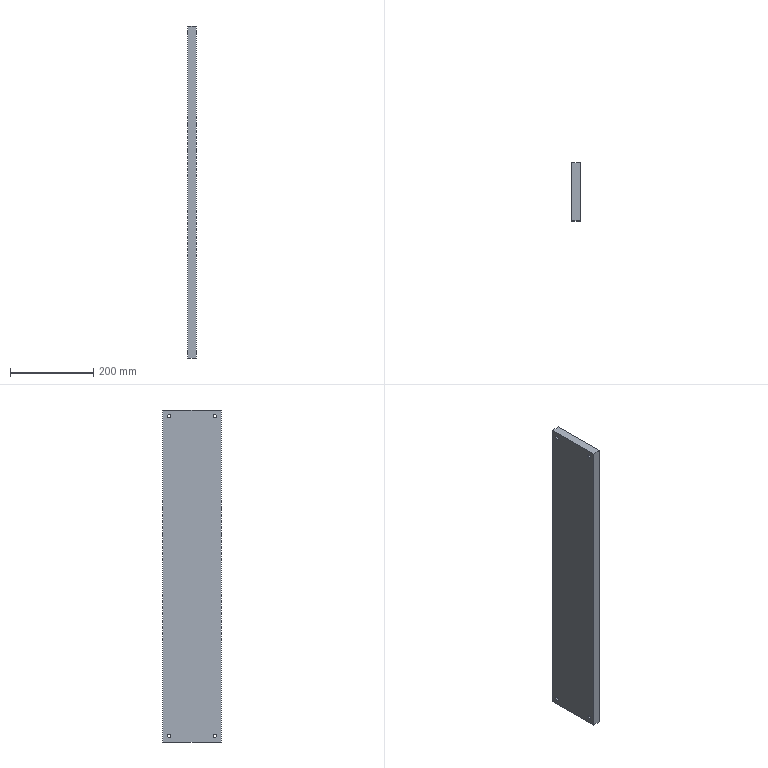Part | STEP file | A14-060 | 1 solid | 14 faces | box 20 x 140 x 800 mm | volume 2235460 mm3 | cylinder 8 | plane 6 | commonest cylinder face diameters 8.5 x8
STEP:
#1=CARTESIAN_POINT('',(0.,0.,0.));
#2=DIRECTION('',(0.,0.,1.));
#3=DIRECTION('',(1.,0.,0.));
#4=AXIS2_PLACEMENT_3D('',#1,#2,#3);
#5=CARTESIAN_POINT('',(-10.,55.,380.75));
#6=VERTEX_POINT('',#5);
#7=CARTESIAN_POINT('',(10.,55.,380.75));
#8=VERTEX_POINT('',#7);
#9=CARTESIAN_POINT('',(-10.,55.,380.75));
#10=DIRECTION('',(1.,0.,0.));
#11=VECTOR('',#10,1.);
#12=LINE('',#9,#11);
#13=CARTESIAN_POINT('',(-10.,55.,385.));
#14=DIRECTION('',(1.,0.,0.));
#15=DIRECTION('',(0.,0.,-1.));
#16=AXIS2_PLACEMENT_3D('',#13,#14,#15);
#17=CYLINDRICAL_SURFACE('',#16,4.25);
#18=CARTESIAN_POINT('',(6.283,0.));
#19=DIRECTION('',(0.,1.));
#20=VECTOR('',#19,1.);
#21=LINE('',#18,#20);
#22=(GEOMETRIC_REPRESENTATION_CONTEXT(2)PARAMETRIC_REPRESENTATION_CONTEXT()REPRESENTATION_CONTEXT('',''));
#23=DEFINITIONAL_REPRESENTATION('',(#21),#22);
#24=PCURVE('',#17,#23);
#25=CARTESIAN_POINT('',(-10.,55.,385.));
#26=DIRECTION('',(1.,0.,0.));
#27=DIRECTION('',(0.,0.,-1.));
#28=AXIS2_PLACEMENT_3D('',#25,#26,#27);
#29=CYLINDRICAL_SURFACE('',#28,4.25);
#30=CARTESIAN_POINT('',(0.,0.));
#31=DIRECTION('',(0.,1.));
#32=VECTOR('',#31,1.);
#33=LINE('',#30,#32);
#34=(GEOMETRIC_REPRESENTATION_CONTEXT(2)PARAMETRIC_REPRESENTATION_CONTEXT()REPRESENTATION_CONTEXT('',''));
#35=DEFINITIONAL_REPRESENTATION('',(#33),#34);
#36=PCURVE('',#29,#35);
#37=SURFACE_CURVE('',#12,(#24,#36),.PCURVE_S1.);
#38=EDGE_CURVE('',#6,#8,#37,.T.);
#39=ORIENTED_EDGE('',*,*,#38,.T.);
#40=CARTESIAN_POINT('',(10.,55.,389.25));
#41=VERTEX_POINT('',#40);
#42=CARTESIAN_POINT('',(10.,55.,385.));
#43=DIRECTION('',(1.,0.,0.));
#44=DIRECTION('',(0.,0.,-1.));
#45=AXIS2_PLACEMENT_3D('',#42,#43,#44);
#46=CIRCLE('',#45,4.25);
#47=CARTESIAN_POINT('',(0.,20.));
#48=DIRECTION('',(1.,0.));
#49=VECTOR('',#48,1.);
#50=LINE('',#47,#49);
#51=(GEOMETRIC_REPRESENTATION_CONTEXT(2)PARAMETRIC_REPRESENTATION_CONTEXT()REPRESENTATION_CONTEXT('',''));
#52=DEFINITIONAL_REPRESENTATION('',(#50),#51);
#53=PCURVE('',#17,#52);
#54=CARTESIAN_POINT('',(10.,0.,0.));
#55=DIRECTION('',(1.,0.,0.));
#56=DIRECTION('',(0.,0.,-1.));
#57=AXIS2_PLACEMENT_3D('',#54,#55,#56);
#58=PLANE('',#57);
#59=CARTESIAN_POINT('',(-385.,55.));
#60=DIRECTION('',(1.,0.));
#61=AXIS2_PLACEMENT_2D('',#59,#60);
#62=CIRCLE('',#61,4.25);
#63=(GEOMETRIC_REPRESENTATION_CONTEXT(2)PARAMETRIC_REPRESENTATION_CONTEXT()REPRESENTATION_CONTEXT('',''));
#64=DEFINITIONAL_REPRESENTATION('',(#62),#63);
#65=PCURVE('',#58,#64);
#66=SURFACE_CURVE('',#46,(#53,#65),.PCURVE_S1.);
#67=EDGE_CURVE('',#41,#8,#66,.T.);
#68=ORIENTED_EDGE('',*,*,#67,.F.);
#69=CARTESIAN_POINT('',(-10.,55.,389.25));
#70=VERTEX_POINT('',#69);
#71=CARTESIAN_POINT('',(-10.,55.,389.25));
#72=DIRECTION('',(1.,0.,0.));
#73=VECTOR('',#72,1.);
#74=LINE('',#71,#73);
#75=CARTESIAN_POINT('',(3.142,0.));
#76=DIRECTION('',(0.,1.));
#77=VECTOR('',#76,1.);
#78=LINE('',#75,#77);
#79=(GEOMETRIC_REPRESENTATION_CONTEXT(2)PARAMETRIC_REPRESENTATION_CONTEXT()REPRESENTATION_CONTEXT('',''));
#80=DEFINITIONAL_REPRESENTATION('',(#78),#79);
#81=PCURVE('',#17,#80);
#82=CARTESIAN_POINT('',(3.142,0.));
#83=DIRECTION('',(0.,1.));
#84=VECTOR('',#83,1.);
#85=LINE('',#82,#84);
#86=(GEOMETRIC_REPRESENTATION_CONTEXT(2)PARAMETRIC_REPRESENTATION_CONTEXT()REPRESENTATION_CONTEXT('',''));
#87=DEFINITIONAL_REPRESENTATION('',(#85),#86);
#88=PCURVE('',#29,#87);
#89=SURFACE_CURVE('',#74,(#81,#88),.PCURVE_S1.);
#90=EDGE_CURVE('',#70,#41,#89,.T.);
#91=ORIENTED_EDGE('',*,*,#90,.F.);
#92=CARTESIAN_POINT('',(-10.,55.,385.));
#93=DIRECTION('',(1.,0.,0.));
#94=DIRECTION('',(0.,0.,-1.));
#95=AXIS2_PLACEMENT_3D('',#92,#93,#94);
#96=CIRCLE('',#95,4.25);
#97=CARTESIAN_POINT('',(0.,0.));
#98=DIRECTION('',(1.,0.));
#99=VECTOR('',#98,1.);
#100=LINE('',#97,#99);
#101=(GEOMETRIC_REPRESENTATION_CONTEXT(2)PARAMETRIC_REPRESENTATION_CONTEXT()REPRESENTATION_CONTEXT('',''));
#102=DEFINITIONAL_REPRESENTATION('',(#100),#101);
#103=PCURVE('',#17,#102);
#104=CARTESIAN_POINT('',(-10.,0.,0.));
#105=DIRECTION('',(1.,0.,0.));
#106=DIRECTION('',(0.,0.,-1.));
#107=AXIS2_PLACEMENT_3D('',#104,#105,#106);
#108=PLANE('',#107);
#109=CARTESIAN_POINT('',(-385.,55.));
#110=DIRECTION('',(1.,0.));
#111=AXIS2_PLACEMENT_2D('',#109,#110);
#112=CIRCLE('',#111,4.25);
#113=(GEOMETRIC_REPRESENTATION_CONTEXT(2)PARAMETRIC_REPRESENTATION_CONTEXT()REPRESENTATION_CONTEXT('',''));
#114=DEFINITIONAL_REPRESENTATION('',(#112),#113);
#115=PCURVE('',#108,#114);
#116=SURFACE_CURVE('',#96,(#103,#115),.PCURVE_S1.);
#117=EDGE_CURVE('',#70,#6,#116,.T.);
#118=ORIENTED_EDGE('',*,*,#117,.T.);
#119=EDGE_LOOP('',(#39,#68,#91,#118));
#120=FACE_BOUND('',#119,.F.);
#121=ADVANCED_FACE('',(#120),#17,.F.);
#122=CARTESIAN_POINT('',(-10.,-55.,380.75));
#123=VERTEX_POINT('',#122);
#124=CARTESIAN_POINT('',(10.,-55.,380.75));
#125=VERTEX_POINT('',#124);
#126=CARTESIAN_POINT('',(-10.,-55.,380.75));
#127=DIRECTION('',(1.,0.,0.));
#128=VECTOR('',#127,1.);
#129=LINE('',#126,#128);
#130=CARTESIAN_POINT('',(-10.,-55.,385.));
#131=DIRECTION('',(1.,0.,0.));
#132=DIRECTION('',(0.,0.,-1.));
#133=AXIS2_PLACEMENT_3D('',#130,#131,#132);
#134=CYLINDRICAL_SURFACE('',#133,4.25);
#135=CARTESIAN_POINT('',(6.283,0.));
#136=DIRECTION('',(0.,1.));
#137=VECTOR('',#136,1.);
#138=LINE('',#135,#137);
#139=(GEOMETRIC_REPRESENTATION_CONTEXT(2)PARAMETRIC_REPRESENTATION_CONTEXT()REPRESENTATION_CONTEXT('',''));
#140=DEFINITIONAL_REPRESENTATION('',(#138),#139);
#141=PCURVE('',#134,#140);
#142=CARTESIAN_POINT('',(-10.,-55.,385.));
#143=DIRECTION('',(1.,0.,0.));
#144=DIRECTION('',(0.,0.,-1.));
#145=AXIS2_PLACEMENT_3D('',#142,#143,#144);
#146=CYLINDRICAL_SURFACE('',#145,4.25);
#147=CARTESIAN_POINT('',(0.,0.));
#148=DIRECTION('',(0.,1.));
#149=VECTOR('',#148,1.);
#150=LINE('',#147,#149);
#151=(GEOMETRIC_REPRESENTATION_CONTEXT(2)PARAMETRIC_REPRESENTATION_CONTEXT()REPRESENTATION_CONTEXT('',''));
#152=DEFINITIONAL_REPRESENTATION('',(#150),#151);
#153=PCURVE('',#146,#152);
#154=SURFACE_CURVE('',#129,(#141,#153),.PCURVE_S1.);
#155=EDGE_CURVE('',#123,#125,#154,.T.);
#156=ORIENTED_EDGE('',*,*,#155,.T.);
#157=CARTESIAN_POINT('',(10.,-55.,389.25));
#158=VERTEX_POINT('',#157);
#159=CARTESIAN_POINT('',(10.,-55.,385.));
#160=DIRECTION('',(1.,0.,0.));
#161=DIRECTION('',(0.,0.,-1.));
#162=AXIS2_PLACEMENT_3D('',#159,#160,#161);
#163=CIRCLE('',#162,4.25);
#164=CARTESIAN_POINT('',(0.,20.));
#165=DIRECTION('',(1.,0.));
#166=VECTOR('',#165,1.);
#167=LINE('',#164,#166);
#168=(GEOMETRIC_REPRESENTATION_CONTEXT(2)PARAMETRIC_REPRESENTATION_CONTEXT()REPRESENTATION_CONTEXT('',''));
#169=DEFINITIONAL_REPRESENTATION('',(#167),#168);
#170=PCURVE('',#134,#169);
#171=CARTESIAN_POINT('',(-385.,-55.));
#172=DIRECTION('',(1.,0.));
#173=AXIS2_PLACEMENT_2D('',#171,#172);
#174=CIRCLE('',#173,4.25);
#175=(GEOMETRIC_REPRESENTATION_CONTEXT(2)PARAMETRIC_REPRESENTATION_CONTEXT()REPRESENTATION_CONTEXT('',''));
#176=DEFINITIONAL_REPRESENTATION('',(#174),#175);
#177=PCURVE('',#58,#176);
#178=SURFACE_CURVE('',#163,(#170,#177),.PCURVE_S1.);
#179=EDGE_CURVE('',#158,#125,#178,.T.);
#180=ORIENTED_EDGE('',*,*,#179,.F.);
#181=CARTESIAN_POINT('',(-10.,-55.,389.25));
#182=VERTEX_POINT('',#181);
#183=CARTESIAN_POINT('',(-10.,-55.,389.25));
#184=DIRECTION('',(1.,0.,0.));
#185=VECTOR('',#184,1.);
#186=LINE('',#183,#185);
#187=CARTESIAN_POINT('',(3.142,0.));
#188=DIRECTION('',(0.,1.));
#189=VECTOR('',#188,1.);
#190=LINE('',#187,#189);
#191=(GEOMETRIC_REPRESENTATION_CONTEXT(2)PARAMETRIC_REPRESENTATION_CONTEXT()REPRESENTATION_CONTEXT('',''));
#192=DEFINITIONAL_REPRESENTATION('',(#190),#191);
#193=PCURVE('',#134,#192);
#194=CARTESIAN_POINT('',(3.142,0.));
#195=DIRECTION('',(0.,1.));
#196=VECTOR('',#195,1.);
#197=LINE('',#194,#196);
#198=(GEOMETRIC_REPRESENTATION_CONTEXT(2)PARAMETRIC_REPRESENTATION_CONTEXT()REPRESENTATION_CONTEXT('',''));
#199=DEFINITIONAL_REPRESENTATION('',(#197),#198);
#200=PCURVE('',#146,#199);
#201=SURFACE_CURVE('',#186,(#193,#200),.PCURVE_S1.);
#202=EDGE_CURVE('',#182,#158,#201,.T.);
#203=ORIENTED_EDGE('',*,*,#202,.F.);
#204=CARTESIAN_POINT('',(-10.,-55.,385.));
#205=DIRECTION('',(1.,0.,0.));
#206=DIRECTION('',(0.,0.,-1.));
#207=AXIS2_PLACEMENT_3D('',#204,#205,#206);
#208=CIRCLE('',#207,4.25);
#209=CARTESIAN_POINT('',(0.,0.));
#210=DIRECTION('',(1.,0.));
#211=VECTOR('',#210,1.);
#212=LINE('',#209,#211);
#213=(GEOMETRIC_REPRESENTATION_CONTEXT(2)PARAMETRIC_REPRESENTATION_CONTEXT()REPRESENTATION_CONTEXT('',''));
#214=DEFINITIONAL_REPRESENTATION('',(#212),#213);
#215=PCURVE('',#134,#214);
#216=CARTESIAN_POINT('',(-385.,-55.));
#217=DIRECTION('',(1.,0.));
#218=AXIS2_PLACEMENT_2D('',#216,#217);
#219=CIRCLE('',#218,4.25);
#220=(GEOMETRIC_REPRESENTATION_CONTEXT(2)PARAMETRIC_REPRESENTATION_CONTEXT()REPRESENTATION_CONTEXT('',''));
#221=DEFINITIONAL_REPRESENTATION('',(#219),#220);
#222=PCURVE('',#108,#221);
#223=SURFACE_CURVE('',#208,(#215,#222),.PCURVE_S1.);
#224=EDGE_CURVE('',#182,#123,#223,.T.);
#225=ORIENTED_EDGE('',*,*,#224,.T.);
#226=EDGE_LOOP('',(#156,#180,#203,#225));
#227=FACE_BOUND('',#226,.F.);
#228=ADVANCED_FACE('',(#227),#134,.F.);
#229=CARTESIAN_POINT('',(-10.,-55.,-389.25));
#230=VERTEX_POINT('',#229);
#231=CARTESIAN_POINT('',(10.,-55.,-389.25));
#232=VERTEX_POINT('',#231);
#233=CARTESIAN_POINT('',(-10.,-55.,-389.25));
#234=DIRECTION('',(1.,0.,0.));
#235=VECTOR('',#234,1.);
#236=LINE('',#233,#235);
#237=CARTESIAN_POINT('',(-10.,-55.,-385.));
#238=DIRECTION('',(1.,0.,0.));
#239=DIRECTION('',(0.,0.,-1.));
#240=AXIS2_PLACEMENT_3D('',#237,#238,#239);
#241=CYLINDRICAL_SURFACE('',#240,4.25);
#242=CARTESIAN_POINT('',(6.283,0.));
#243=DIRECTION('',(0.,1.));
#244=VECTOR('',#243,1.);
#245=LINE('',#242,#244);
#246=(GEOMETRIC_REPRESENTATION_CONTEXT(2)PARAMETRIC_REPRESENTATION_CONTEXT()REPRESENTATION_CONTEXT('',''));
#247=DEFINITIONAL_REPRESENTATION('',(#245),#246);
#248=PCURVE('',#241,#247);
#249=CARTESIAN_POINT('',(-10.,-55.,-385.));
#250=DIRECTION('',(1.,0.,0.));
#251=DIRECTION('',(0.,0.,-1.));
#252=AXIS2_PLACEMENT_3D('',#249,#250,#251);
#253=CYLINDRICAL_SURFACE('',#252,4.25);
#254=CARTESIAN_POINT('',(0.,0.));
#255=DIRECTION('',(0.,1.));
#256=VECTOR('',#255,1.);
#257=LINE('',#254,#256);
#258=(GEOMETRIC_REPRESENTATION_CONTEXT(2)PARAMETRIC_REPRESENTATION_CONTEXT()REPRESENTATION_CONTEXT('',''));
#259=DEFINITIONAL_REPRESENTATION('',(#257),#258);
#260=PCURVE('',#253,#259);
#261=SURFACE_CURVE('',#236,(#248,#260),.PCURVE_S1.);
#262=EDGE_CURVE('',#230,#232,#261,.T.);
#263=ORIENTED_EDGE('',*,*,#262,.T.);
#264=CARTESIAN_POINT('',(10.,-55.,-380.75));
#265=VERTEX_POINT('',#264);
#266=CARTESIAN_POINT('',(10.,-55.,-385.));
#267=DIRECTION('',(1.,0.,0.));
#268=DIRECTION('',(0.,0.,-1.));
#269=AXIS2_PLACEMENT_3D('',#266,#267,#268);
#270=CIRCLE('',#269,4.25);
#271=CARTESIAN_POINT('',(0.,20.));
#272=DIRECTION('',(1.,0.));
#273=VECTOR('',#272,1.);
#274=LINE('',#271,#273);
#275=(GEOMETRIC_REPRESENTATION_CONTEXT(2)PARAMETRIC_REPRESENTATION_CONTEXT()REPRESENTATION_CONTEXT('',''));
#276=DEFINITIONAL_REPRESENTATION('',(#274),#275);
#277=PCURVE('',#241,#276);
#278=CARTESIAN_POINT('',(385.,-55.));
#279=DIRECTION('',(1.,0.));
#280=AXIS2_PLACEMENT_2D('',#278,#279);
#281=CIRCLE('',#280,4.25);
#282=(GEOMETRIC_REPRESENTATION_CONTEXT(2)PARAMETRIC_REPRESENTATION_CONTEXT()REPRESENTATION_CONTEXT('',''));
#283=DEFINITIONAL_REPRESENTATION('',(#281),#282);
#284=PCURVE('',#58,#283);
#285=SURFACE_CURVE('',#270,(#277,#284),.PCURVE_S1.);
#286=EDGE_CURVE('',#265,#232,#285,.T.);
#287=ORIENTED_EDGE('',*,*,#286,.F.);
#288=CARTESIAN_POINT('',(-10.,-55.,-380.75));
#289=VERTEX_POINT('',#288);
#290=CARTESIAN_POINT('',(-10.,-55.,-380.75));
#291=DIRECTION('',(1.,0.,0.));
#292=VECTOR('',#291,1.);
#293=LINE('',#290,#292);
#294=CARTESIAN_POINT('',(3.142,0.));
#295=DIRECTION('',(0.,1.));
#296=VECTOR('',#295,1.);
#297=LINE('',#294,#296);
#298=(GEOMETRIC_REPRESENTATION_CONTEXT(2)PARAMETRIC_REPRESENTATION_CONTEXT()REPRESENTATION_CONTEXT('',''));
#299=DEFINITIONAL_REPRESENTATION('',(#297),#298);
#300=PCURVE('',#241,#299);
#301=CARTESIAN_POINT('',(3.142,0.));
#302=DIRECTION('',(0.,1.));
#303=VECTOR('',#302,1.);
#304=LINE('',#301,#303);
#305=(GEOMETRIC_REPRESENTATION_CONTEXT(2)PARAMETRIC_REPRESENTATION_CONTEXT()REPRESENTATION_CONTEXT('',''));
#306=DEFINITIONAL_REPRESENTATION('',(#304),#305);
#307=PCURVE('',#253,#306);
#308=SURFACE_CURVE('',#293,(#300,#307),.PCURVE_S1.);
#309=EDGE_CURVE('',#289,#265,#308,.T.);
#310=ORIENTED_EDGE('',*,*,#309,.F.);
#311=CARTESIAN_POINT('',(-10.,-55.,-385.));
#312=DIRECTION('',(1.,0.,0.));
#313=DIRECTION('',(0.,0.,-1.));
#314=AXIS2_PLACEMENT_3D('',#311,#312,#313);
#315=CIRCLE('',#314,4.25);
#316=CARTESIAN_POINT('',(0.,0.));
#317=DIRECTION('',(1.,0.));
#318=VECTOR('',#317,1.);
#319=LINE('',#316,#318);
#320=(GEOMETRIC_REPRESENTATION_CONTEXT(2)PARAMETRIC_REPRESENTATION_CONTEXT()REPRESENTATION_CONTEXT('',''));
#321=DEFINITIONAL_REPRESENTATION('',(#319),#320);
#322=PCURVE('',#241,#321);
#323=CARTESIAN_POINT('',(385.,-55.));
#324=DIRECTION('',(1.,0.));
#325=AXIS2_PLACEMENT_2D('',#323,#324);
#326=CIRCLE('',#325,4.25);
#327=(GEOMETRIC_REPRESENTATION_CONTEXT(2)PARAMETRIC_REPRESENTATION_CONTEXT()REPRESENTATION_CONTEXT('',''));
#328=DEFINITIONAL_REPRESENTATION('',(#326),#327);
#329=PCURVE('',#108,#328);
#330=SURFACE_CURVE('',#315,(#322,#329),.PCURVE_S1.);
#331=EDGE_CURVE('',#289,#230,#330,.T.);
#332=ORIENTED_EDGE('',*,*,#331,.T.);
#333=EDGE_LOOP('',(#263,#287,#310,#332));
#334=FACE_BOUND('',#333,.F.);
#335=ADVANCED_FACE('',(#334),#241,.F.);
#336=CARTESIAN_POINT('',(-10.,55.,-389.25));
#337=VERTEX_POINT('',#336);
#338=CARTESIAN_POINT('',(10.,55.,-389.25));
#339=VERTEX_POINT('',#338);
#340=CARTESIAN_POINT('',(-10.,55.,-389.25));
#341=DIRECTION('',(1.,0.,0.));
#342=VECTOR('',#341,1.);
#343=LINE('',#340,#342);
#344=CARTESIAN_POINT('',(-10.,55.,-385.));
#345=DIRECTION('',(1.,0.,0.));
#346=DIRECTION('',(0.,0.,-1.));
#347=AXIS2_PLACEMENT_3D('',#344,#345,#346);
#348=CYLINDRICAL_SURFACE('',#347,4.25);
#349=CARTESIAN_POINT('',(6.283,0.));
#350=DIRECTION('',(0.,1.));
#351=VECTOR('',#350,1.);
#352=LINE('',#349,#351);
#353=(GEOMETRIC_REPRESENTATION_CONTEXT(2)PARAMETRIC_REPRESENTATION_CONTEXT()REPRESENTATION_CONTEXT('',''));
#354=DEFINITIONAL_REPRESENTATION('',(#352),#353);
#355=PCURVE('',#348,#354);
#356=CARTESIAN_POINT('',(-10.,55.,-385.));
#357=DIRECTION('',(1.,0.,0.));
#358=DIRECTION('',(0.,0.,-1.));
#359=AXIS2_PLACEMENT_3D('',#356,#357,#358);
#360=CYLINDRICAL_SURFACE('',#359,4.25);
#361=CARTESIAN_POINT('',(0.,0.));
#362=DIRECTION('',(0.,1.));
#363=VECTOR('',#362,1.);
#364=LINE('',#361,#363);
#365=(GEOMETRIC_REPRESENTATION_CONTEXT(2)PARAMETRIC_REPRESENTATION_CONTEXT()REPRESENTATION_CONTEXT('',''));
#366=DEFINITIONAL_REPRESENTATION('',(#364),#365);
#367=PCURVE('',#360,#366);
#368=SURFACE_CURVE('',#343,(#355,#367),.PCURVE_S1.);
#369=EDGE_CURVE('',#337,#339,#368,.T.);
#370=ORIENTED_EDGE('',*,*,#369,.T.);
#371=CARTESIAN_POINT('',(10.,55.,-380.75));
#372=VERTEX_POINT('',#371);
#373=CARTESIAN_POINT('',(10.,55.,-385.));
#374=DIRECTION('',(1.,0.,0.));
#375=DIRECTION('',(0.,0.,-1.));
#376=AXIS2_PLACEMENT_3D('',#373,#374,#375);
#377=CIRCLE('',#376,4.25);
#378=CARTESIAN_POINT('',(0.,20.));
#379=DIRECTION('',(1.,0.));
#380=VECTOR('',#379,1.);
#381=LINE('',#378,#380);
#382=(GEOMETRIC_REPRESENTATION_CONTEXT(2)PARAMETRIC_REPRESENTATION_CONTEXT()REPRESENTATION_CONTEXT('',''));
#383=DEFINITIONAL_REPRESENTATION('',(#381),#382);
#384=PCURVE('',#348,#383);
#385=CARTESIAN_POINT('',(385.,55.));
#386=DIRECTION('',(1.,0.));
#387=AXIS2_PLACEMENT_2D('',#385,#386);
#388=CIRCLE('',#387,4.25);
#389=(GEOMETRIC_REPRESENTATION_CONTEXT(2)PARAMETRIC_REPRESENTATION_CONTEXT()REPRESENTATION_CONTEXT('',''));
#390=DEFINITIONAL_REPRESENTATION('',(#388),#389);
#391=PCURVE('',#58,#390);
#392=SURFACE_CURVE('',#377,(#384,#391),.PCURVE_S1.);
#393=EDGE_CURVE('',#372,#339,#392,.T.);
#394=ORIENTED_EDGE('',*,*,#393,.F.);
#395=CARTESIAN_POINT('',(-10.,55.,-380.75));
#396=VERTEX_POINT('',#395);
#397=CARTESIAN_POINT('',(-10.,55.,-380.75));
#398=DIRECTION('',(1.,0.,0.));
#399=VECTOR('',#398,1.);
#400=LINE('',#397,#399);
#401=CARTESIAN_POINT('',(3.142,0.));
#402=DIRECTION('',(0.,1.));
#403=VECTOR('',#402,1.);
#404=LINE('',#401,#403);
#405=(GEOMETRIC_REPRESENTATION_CONTEXT(2)PARAMETRIC_REPRESENTATION_CONTEXT()REPRESENTATION_CONTEXT('',''));
#406=DEFINITIONAL_REPRESENTATION('',(#404),#405);
#407=PCURVE('',#348,#406);
#408=CARTESIAN_POINT('',(3.142,0.));
#409=DIRECTION('',(0.,1.));
#410=VECTOR('',#409,1.);
#411=LINE('',#408,#410);
#412=(GEOMETRIC_REPRESENTATION_CONTEXT(2)PARAMETRIC_REPRESENTATION_CONTEXT()REPRESENTATION_CONTEXT('',''));
#413=DEFINITIONAL_REPRESENTATION('',(#411),#412);
#414=PCURVE('',#360,#413);
#415=SURFACE_CURVE('',#400,(#407,#414),.PCURVE_S1.);
#416=EDGE_CURVE('',#396,#372,#415,.T.);
#417=ORIENTED_EDGE('',*,*,#416,.F.);
#418=CARTESIAN_POINT('',(-10.,55.,-385.));
#419=DIRECTION('',(1.,0.,0.));
#420=DIRECTION('',(0.,0.,-1.));
#421=AXIS2_PLACEMENT_3D('',#418,#419,#420);
#422=CIRCLE('',#421,4.25);
#423=CARTESIAN_POINT('',(0.,0.));
#424=DIRECTION('',(1.,0.));
#425=VECTOR('',#424,1.);
#426=LINE('',#423,#425);
#427=(GEOMETRIC_REPRESENTATION_CONTEXT(2)PARAMETRIC_REPRESENTATION_CONTEXT()REPRESENTATION_CONTEXT('',''));
#428=DEFINITIONAL_REPRESENTATION('',(#426),#427);
#429=PCURVE('',#348,#428);
#430=CARTESIAN_POINT('',(385.,55.));
#431=DIRECTION('',(1.,0.));
#432=AXIS2_PLACEMENT_2D('',#430,#431);
#433=CIRCLE('',#432,4.25);
#434=(GEOMETRIC_REPRESENTATION_CONTEXT(2)PARAMETRIC_REPRESENTATION_CONTEXT()REPRESENTATION_CONTEXT('',''));
#435=DEFINITIONAL_REPRESENTATION('',(#433),#434);
#436=PCURVE('',#108,#435);
#437=SURFACE_CURVE('',#422,(#429,#436),.PCURVE_S1.);
#438=EDGE_CURVE('',#396,#337,#437,.T.);
#439=ORIENTED_EDGE('',*,*,#438,.T.);
#440=EDGE_LOOP('',(#370,#394,#417,#439));
#441=FACE_BOUND('',#440,.F.);
#442=ADVANCED_FACE('',(#441),#348,.F.);
#443=CARTESIAN_POINT('',(-10.,-70.,-400.));
#444=VERTEX_POINT('',#443);
#445=CARTESIAN_POINT('',(-10.,70.,-400.));
#446=VERTEX_POINT('',#445);
#447=CARTESIAN_POINT('',(-10.,70.,-400.));
#448=DIRECTION('',(0.,1.,0.));
#449=VECTOR('',#448,1.);
#450=LINE('',#447,#449);
#451=CARTESIAN_POINT('',(10.,70.,-400.));
#452=DIRECTION('',(0.,0.,1.));
#453=DIRECTION('',(1.,0.,0.));
#454=AXIS2_PLACEMENT_3D('',#451,#452,#453);
#455=PLANE('',#454);
#456=CARTESIAN_POINT('',(-20.,0.));
#457=DIRECTION('',(0.,1.));
#458=VECTOR('',#457,1.);
#459=LINE('',#456,#458);
#460=(GEOMETRIC_REPRESENTATION_CONTEXT(2)PARAMETRIC_REPRESENTATION_CONTEXT()REPRESENTATION_CONTEXT('',''));
#461=DEFINITIONAL_REPRESENTATION('',(#459),#460);
#462=PCURVE('',#455,#461);
#463=CARTESIAN_POINT('',(400.,70.));
#464=DIRECTION('',(0.,1.));
#465=VECTOR('',#464,1.);
#466=LINE('',#463,#465);
#467=(GEOMETRIC_REPRESENTATION_CONTEXT(2)PARAMETRIC_REPRESENTATION_CONTEXT()REPRESENTATION_CONTEXT('',''));
#468=DEFINITIONAL_REPRESENTATION('',(#466),#467);
#469=PCURVE('',#108,#468);
#470=SURFACE_CURVE('',#450,(#462,#469),.PCURVE_S1.);
#471=EDGE_CURVE('',#444,#446,#470,.T.);
#472=ORIENTED_EDGE('',*,*,#471,.T.);
#473=CARTESIAN_POINT('',(10.,70.,-400.));
#474=VERTEX_POINT('',#473);
#475=CARTESIAN_POINT('',(10.,70.,-400.));
#476=DIRECTION('',(-1.,0.,0.));
#477=VECTOR('',#476,1.);
#478=LINE('',#475,#477);
#479=CARTESIAN_POINT('',(0.,0.));
#480=DIRECTION('',(-1.,0.));
#481=VECTOR('',#480,1.);
#482=LINE('',#479,#481);
#483=(GEOMETRIC_REPRESENTATION_CONTEXT(2)PARAMETRIC_REPRESENTATION_CONTEXT()REPRESENTATION_CONTEXT('',''));
#484=DEFINITIONAL_REPRESENTATION('',(#482),#483);
#485=PCURVE('',#455,#484);
#486=CARTESIAN_POINT('',(10.,70.,400.));
#487=DIRECTION('',(0.,-1.,0.));
#488=DIRECTION('',(0.,0.,-1.));
#489=AXIS2_PLACEMENT_3D('',#486,#487,#488);
#490=PLANE('',#489);
#491=CARTESIAN_POINT('',(800.,0.));
#492=DIRECTION('',(0.,-1.));
#493=VECTOR('',#492,1.);
#494=LINE('',#491,#493);
#495=(GEOMETRIC_REPRESENTATION_CONTEXT(2)PARAMETRIC_REPRESENTATION_CONTEXT()REPRESENTATION_CONTEXT('',''));
#496=DEFINITIONAL_REPRESENTATION('',(#494),#495);
#497=PCURVE('',#490,#496);
#498=SURFACE_CURVE('',#478,(#485,#497),.PCURVE_S1.);
#499=EDGE_CURVE('',#474,#446,#498,.T.);
#500=ORIENTED_EDGE('',*,*,#499,.F.);
#501=CARTESIAN_POINT('',(10.,-70.,-400.));
#502=VERTEX_POINT('',#501);
#503=CARTESIAN_POINT('',(10.,70.,-400.));
#504=DIRECTION('',(0.,1.,0.));
#505=VECTOR('',#504,1.);
#506=LINE('',#503,#505);
#507=CARTESIAN_POINT('',(0.,0.));
#508=DIRECTION('',(0.,1.));
#509=VECTOR('',#508,1.);
#510=LINE('',#507,#509);
#511=(GEOMETRIC_REPRESENTATION_CONTEXT(2)PARAMETRIC_REPRESENTATION_CONTEXT()REPRESENTATION_CONTEXT('',''));
#512=DEFINITIONAL_REPRESENTATION('',(#510),#511);
#513=PCURVE('',#455,#512);
#514=CARTESIAN_POINT('',(400.,70.));
#515=DIRECTION('',(0.,1.));
#516=VECTOR('',#515,1.);
#517=LINE('',#514,#516);
#518=(GEOMETRIC_REPRESENTATION_CONTEXT(2)PARAMETRIC_REPRESENTATION_CONTEXT()REPRESENTATION_CONTEXT('',''));
#519=DEFINITIONAL_REPRESENTATION('',(#517),#518);
#520=PCURVE('',#58,#519);
#521=SURFACE_CURVE('',#506,(#513,#520),.PCURVE_S1.);
#522=EDGE_CURVE('',#502,#474,#521,.T.);
#523=ORIENTED_EDGE('',*,*,#522,.F.);
#524=CARTESIAN_POINT('',(10.,-70.,-400.));
#525=DIRECTION('',(-1.,0.,0.));
#526=VECTOR('',#525,1.);
#527=LINE('',#524,#526);
#528=CARTESIAN_POINT('',(0.,-140.));
#529=DIRECTION('',(-1.,0.));
#530=VECTOR('',#529,1.);
#531=LINE('',#528,#530);
#532=(GEOMETRIC_REPRESENTATION_CONTEXT(2)PARAMETRIC_REPRESENTATION_CONTEXT()REPRESENTATION_CONTEXT('',''));
#533=DEFINITIONAL_REPRESENTATION('',(#531),#532);
#534=PCURVE('',#455,#533);
#535=CARTESIAN_POINT('',(10.,-70.,400.));
#536=DIRECTION('',(0.,1.,0.));
#537=DIRECTION('',(0.,0.,1.));
#538=AXIS2_PLACEMENT_3D('',#535,#536,#537);
#539=PLANE('',#538);
#540=CARTESIAN_POINT('',(-800.,0.));
#541=DIRECTION('',(0.,-1.));
#542=VECTOR('',#541,1.);
#543=LINE('',#540,#542);
#544=(GEOMETRIC_REPRESENTATION_CONTEXT(2)PARAMETRIC_REPRESENTATION_CONTEXT()REPRESENTATION_CONTEXT('',''));
#545=DEFINITIONAL_REPRESENTATION('',(#543),#544);
#546=PCURVE('',#539,#545);
#547=SURFACE_CURVE('',#527,(#534,#546),.PCURVE_S1.);
#548=EDGE_CURVE('',#502,#444,#547,.T.);
#549=ORIENTED_EDGE('',*,*,#548,.T.);
#550=EDGE_LOOP('',(#472,#500,#523,#549));
#551=FACE_BOUND('',#550,.T.);
#552=ADVANCED_FACE('',(#551),#455,.F.);
#553=CARTESIAN_POINT('',(-10.,70.,400.));
#554=VERTEX_POINT('',#553);
#555=CARTESIAN_POINT('',(-10.,70.,400.));
#556=DIRECTION('',(0.,0.,1.));
#557=VECTOR('',#556,1.);
#558=LINE('',#555,#557);
#559=CARTESIAN_POINT('',(0.,-20.));
#560=DIRECTION('',(-1.,0.));
#561=VECTOR('',#560,1.);
#562=LINE('',#559,#561);
#563=(GEOMETRIC_REPRESENTATION_CONTEXT(2)PARAMETRIC_REPRESENTATION_CONTEXT()REPRESENTATION_CONTEXT('',''));
#564=DEFINITIONAL_REPRESENTATION('',(#562),#563);
#565=PCURVE('',#490,#564);
#566=CARTESIAN_POINT('',(-400.,70.));
#567=DIRECTION('',(-1.,0.));
#568=VECTOR('',#567,1.);
#569=LINE('',#566,#568);
#570=(GEOMETRIC_REPRESENTATION_CONTEXT(2)PARAMETRIC_REPRESENTATION_CONTEXT()REPRESENTATION_CONTEXT('',''));
#571=DEFINITIONAL_REPRESENTATION('',(#569),#570);
#572=PCURVE('',#108,#571);
#573=SURFACE_CURVE('',#558,(#565,#572),.PCURVE_S1.);
#574=EDGE_CURVE('',#446,#554,#573,.T.);
#575=ORIENTED_EDGE('',*,*,#574,.T.);
#576=CARTESIAN_POINT('',(10.,70.,400.));
#577=VERTEX_POINT('',#576);
#578=CARTESIAN_POINT('',(10.,70.,400.));
#579=DIRECTION('',(-1.,0.,0.));
#580=VECTOR('',#579,1.);
#581=LINE('',#578,#580);
#582=CARTESIAN_POINT('',(0.,0.));
#583=DIRECTION('',(0.,-1.));
#584=VECTOR('',#583,1.);
#585=LINE('',#582,#584);
#586=(GEOMETRIC_REPRESENTATION_CONTEXT(2)PARAMETRIC_REPRESENTATION_CONTEXT()REPRESENTATION_CONTEXT('',''));
#587=DEFINITIONAL_REPRESENTATION('',(#585),#586);
#588=PCURVE('',#490,#587);
#589=CARTESIAN_POINT('',(10.,70.,400.));
#590=DIRECTION('',(0.,0.,-1.));
#591=DIRECTION('',(-1.,0.,0.));
#592=AXIS2_PLACEMENT_3D('',#589,#590,#591);
#593=PLANE('',#592);
#594=CARTESIAN_POINT('',(0.,0.));
#595=DIRECTION('',(1.,0.));
#596=VECTOR('',#595,1.);
#597=LINE('',#594,#596);
#598=(GEOMETRIC_REPRESENTATION_CONTEXT(2)PARAMETRIC_REPRESENTATION_CONTEXT()REPRESENTATION_CONTEXT('',''));
#599=DEFINITIONAL_REPRESENTATION('',(#597),#598);
#600=PCURVE('',#593,#599);
#601=SURFACE_CURVE('',#581,(#588,#600),.PCURVE_S1.);
#602=EDGE_CURVE('',#577,#554,#601,.T.);
#603=ORIENTED_EDGE('',*,*,#602,.F.);
#604=CARTESIAN_POINT('',(10.,70.,400.));
#605=DIRECTION('',(0.,0.,1.));
#606=VECTOR('',#605,1.);
#607=LINE('',#604,#606);
#608=CARTESIAN_POINT('',(0.,0.));
#609=DIRECTION('',(-1.,0.));
#610=VECTOR('',#609,1.);
#611=LINE('',#608,#610);
#612=(GEOMETRIC_REPRESENTATION_CONTEXT(2)PARAMETRIC_REPRESENTATION_CONTEXT()REPRESENTATION_CONTEXT('',''));
#613=DEFINITIONAL_REPRESENTATION('',(#611),#612);
#614=PCURVE('',#490,#613);
#615=CARTESIAN_POINT('',(-400.,70.));
#616=DIRECTION('',(-1.,0.));
#617=VECTOR('',#616,1.);
#618=LINE('',#615,#617);
#619=(GEOMETRIC_REPRESENTATION_CONTEXT(2)PARAMETRIC_REPRESENTATION_CONTEXT()REPRESENTATION_CONTEXT('',''));
#620=DEFINITIONAL_REPRESENTATION('',(#618),#619);
#621=PCURVE('',#58,#620);
#622=SURFACE_CURVE('',#607,(#614,#621),.PCURVE_S1.);
#623=EDGE_CURVE('',#474,#577,#622,.T.);
#624=ORIENTED_EDGE('',*,*,#623,.F.);
#625=ORIENTED_EDGE('',*,*,#499,.T.);
#626=EDGE_LOOP('',(#575,#603,#624,#625));
#627=FACE_BOUND('',#626,.T.);
#628=ADVANCED_FACE('',(#627),#490,.F.);
#629=CARTESIAN_POINT('',(-10.,-70.,400.));
#630=VERTEX_POINT('',#629);
#631=CARTESIAN_POINT('',(-10.,70.,400.));
#632=DIRECTION('',(0.,-1.,0.));
#633=VECTOR('',#632,1.);
#634=LINE('',#631,#633);
#635=CARTESIAN_POINT('',(20.,0.));
#636=DIRECTION('',(0.,-1.));
#637=VECTOR('',#636,1.);
#638=LINE('',#635,#637);
#639=(GEOMETRIC_REPRESENTATION_CONTEXT(2)PARAMETRIC_REPRESENTATION_CONTEXT()REPRESENTATION_CONTEXT('',''));
#640=DEFINITIONAL_REPRESENTATION('',(#638),#639);
#641=PCURVE('',#593,#640);
#642=CARTESIAN_POINT('',(-400.,70.));
#643=DIRECTION('',(0.,-1.));
#644=VECTOR('',#643,1.);
#645=LINE('',#642,#644);
#646=(GEOMETRIC_REPRESENTATION_CONTEXT(2)PARAMETRIC_REPRESENTATION_CONTEXT()REPRESENTATION_CONTEXT('',''));
#647=DEFINITIONAL_REPRESENTATION('',(#645),#646);
#648=PCURVE('',#108,#647);
#649=SURFACE_CURVE('',#634,(#641,#648),.PCURVE_S1.);
#650=EDGE_CURVE('',#554,#630,#649,.T.);
#651=ORIENTED_EDGE('',*,*,#650,.T.);
#652=CARTESIAN_POINT('',(10.,-70.,400.));
#653=VERTEX_POINT('',#652);
#654=CARTESIAN_POINT('',(10.,-70.,400.));
#655=DIRECTION('',(-1.,0.,0.));
#656=VECTOR('',#655,1.);
#657=LINE('',#654,#656);
#658=CARTESIAN_POINT('',(0.,-140.));
#659=DIRECTION('',(1.,0.));
#660=VECTOR('',#659,1.);
#661=LINE('',#658,#660);
#662=(GEOMETRIC_REPRESENTATION_CONTEXT(2)PARAMETRIC_REPRESENTATION_CONTEXT()REPRESENTATION_CONTEXT('',''));
#663=DEFINITIONAL_REPRESENTATION('',(#661),#662);
#664=PCURVE('',#593,#663);
#665=CARTESIAN_POINT('',(0.,0.));
#666=DIRECTION('',(0.,-1.));
#667=VECTOR('',#666,1.);
#668=LINE('',#665,#667);
#669=(GEOMETRIC_REPRESENTATION_CONTEXT(2)PARAMETRIC_REPRESENTATION_CONTEXT()REPRESENTATION_CONTEXT('',''));
#670=DEFINITIONAL_REPRESENTATION('',(#668),#669);
#671=PCURVE('',#539,#670);
#672=SURFACE_CURVE('',#657,(#664,#671),.PCURVE_S1.);
#673=EDGE_CURVE('',#653,#630,#672,.T.);
#674=ORIENTED_EDGE('',*,*,#673,.F.);
#675=CARTESIAN_POINT('',(10.,70.,400.));
#676=DIRECTION('',(0.,-1.,0.));
#677=VECTOR('',#676,1.);
#678=LINE('',#675,#677);
#679=CARTESIAN_POINT('',(0.,0.));
#680=DIRECTION('',(0.,-1.));
#681=VECTOR('',#680,1.);
#682=LINE('',#679,#681);
#683=(GEOMETRIC_REPRESENTATION_CONTEXT(2)PARAMETRIC_REPRESENTATION_CONTEXT()REPRESENTATION_CONTEXT('',''));
#684=DEFINITIONAL_REPRESENTATION('',(#682),#683);
#685=PCURVE('',#593,#684);
#686=CARTESIAN_POINT('',(-400.,70.));
#687=DIRECTION('',(0.,-1.));
#688=VECTOR('',#687,1.);
#689=LINE('',#686,#688);
#690=(GEOMETRIC_REPRESENTATION_CONTEXT(2)PARAMETRIC_REPRESENTATION_CONTEXT()REPRESENTATION_CONTEXT('',''));
#691=DEFINITIONAL_REPRESENTATION('',(#689),#690);
#692=PCURVE('',#58,#691);
#693=SURFACE_CURVE('',#678,(#685,#692),.PCURVE_S1.);
#694=EDGE_CURVE('',#577,#653,#693,.T.);
#695=ORIENTED_EDGE('',*,*,#694,.F.);
#696=ORIENTED_EDGE('',*,*,#602,.T.);
#697=EDGE_LOOP('',(#651,#674,#695,#696));
#698=FACE_BOUND('',#697,.T.);
#699=ADVANCED_FACE('',(#698),#593,.F.);
#700=CARTESIAN_POINT('',(-10.,-70.,400.));
#701=DIRECTION('',(0.,0.,-1.));
#702=VECTOR('',#701,1.);
#703=LINE('',#700,#702);
#704=CARTESIAN_POINT('',(0.,-20.));
#705=DIRECTION('',(-1.,0.));
#706=VECTOR('',#705,1.);
#707=LINE('',#704,#706);
#708=(GEOMETRIC_REPRESENTATION_CONTEXT(2)PARAMETRIC_REPRESENTATION_CONTEXT()REPRESENTATION_CONTEXT('',''));
#709=DEFINITIONAL_REPRESENTATION('',(#707),#708);
#710=PCURVE('',#539,#709);
#711=CARTESIAN_POINT('',(-400.,-70.));
#712=DIRECTION('',(1.,0.));
#713=VECTOR('',#712,1.);
#714=LINE('',#711,#713);
#715=(GEOMETRIC_REPRESENTATION_CONTEXT(2)PARAMETRIC_REPRESENTATION_CONTEXT()REPRESENTATION_CONTEXT('',''));
#716=DEFINITIONAL_REPRESENTATION('',(#714),#715);
#717=PCURVE('',#108,#716);
#718=SURFACE_CURVE('',#703,(#710,#717),.PCURVE_S1.);
#719=EDGE_CURVE('',#630,#444,#718,.T.);
#720=ORIENTED_EDGE('',*,*,#719,.T.);
#721=ORIENTED_EDGE('',*,*,#548,.F.);
#722=CARTESIAN_POINT('',(10.,-70.,400.));
#723=DIRECTION('',(0.,0.,-1.));
#724=VECTOR('',#723,1.);
#725=LINE('',#722,#724);
#726=CARTESIAN_POINT('',(0.,0.));
#727=DIRECTION('',(-1.,0.));
#728=VECTOR('',#727,1.);
#729=LINE('',#726,#728);
#730=(GEOMETRIC_REPRESENTATION_CONTEXT(2)PARAMETRIC_REPRESENTATION_CONTEXT()REPRESENTATION_CONTEXT('',''));
#731=DEFINITIONAL_REPRESENTATION('',(#729),#730);
#732=PCURVE('',#539,#731);
#733=CARTESIAN_POINT('',(-400.,-70.));
#734=DIRECTION('',(1.,0.));
#735=VECTOR('',#734,1.);
#736=LINE('',#733,#735);
#737=(GEOMETRIC_REPRESENTATION_CONTEXT(2)PARAMETRIC_REPRESENTATION_CONTEXT()REPRESENTATION_CONTEXT('',''));
#738=DEFINITIONAL_REPRESENTATION('',(#736),#737);
#739=PCURVE('',#58,#738);
#740=SURFACE_CURVE('',#725,(#732,#739),.PCURVE_S1.);
#741=EDGE_CURVE('',#653,#502,#740,.T.);
#742=ORIENTED_EDGE('',*,*,#741,.F.);
#743=ORIENTED_EDGE('',*,*,#673,.T.);
#744=EDGE_LOOP('',(#720,#721,#742,#743));
#745=FACE_BOUND('',#744,.T.);
#746=ADVANCED_FACE('',(#745),#539,.F.);
#747=CARTESIAN_POINT('',(10.,55.,385.));
#748=DIRECTION('',(1.,0.,0.));
#749=DIRECTION('',(0.,0.,-1.));
#750=AXIS2_PLACEMENT_3D('',#747,#748,#749);
#751=CIRCLE('',#750,4.25);
#752=CARTESIAN_POINT('',(-385.,55.));
#753=DIRECTION('',(1.,0.));
#754=AXIS2_PLACEMENT_2D('',#752,#753);
#755=CIRCLE('',#754,4.25);
#756=(GEOMETRIC_REPRESENTATION_CONTEXT(2)PARAMETRIC_REPRESENTATION_CONTEXT()REPRESENTATION_CONTEXT('',''));
#757=DEFINITIONAL_REPRESENTATION('',(#755),#756);
#758=PCURVE('',#58,#757);
#759=CARTESIAN_POINT('',(0.,20.));
#760=DIRECTION('',(1.,0.));
#761=VECTOR('',#760,1.);
#762=LINE('',#759,#761);
#763=(GEOMETRIC_REPRESENTATION_CONTEXT(2)PARAMETRIC_REPRESENTATION_CONTEXT()REPRESENTATION_CONTEXT('',''));
#764=DEFINITIONAL_REPRESENTATION('',(#762),#763);
#765=PCURVE('',#29,#764);
#766=SURFACE_CURVE('',#751,(#758,#765),.PCURVE_S1.);
#767=EDGE_CURVE('',#8,#41,#766,.T.);
#768=ORIENTED_EDGE('',*,*,#767,.F.);
#769=ORIENTED_EDGE('',*,*,#67,.F.);
#770=EDGE_LOOP('',(#768,#769));
#771=FACE_BOUND('',#770,.T.);
#772=CARTESIAN_POINT('',(10.,-55.,385.));
#773=DIRECTION('',(1.,0.,0.));
#774=DIRECTION('',(0.,0.,-1.));
#775=AXIS2_PLACEMENT_3D('',#772,#773,#774);
#776=CIRCLE('',#775,4.25);
#777=CARTESIAN_POINT('',(-385.,-55.));
#778=DIRECTION('',(1.,0.));
#779=AXIS2_PLACEMENT_2D('',#777,#778);
#780=CIRCLE('',#779,4.25);
#781=(GEOMETRIC_REPRESENTATION_CONTEXT(2)PARAMETRIC_REPRESENTATION_CONTEXT()REPRESENTATION_CONTEXT('',''));
#782=DEFINITIONAL_REPRESENTATION('',(#780),#781);
#783=PCURVE('',#58,#782);
#784=CARTESIAN_POINT('',(0.,20.));
#785=DIRECTION('',(1.,0.));
#786=VECTOR('',#785,1.);
#787=LINE('',#784,#786);
#788=(GEOMETRIC_REPRESENTATION_CONTEXT(2)PARAMETRIC_REPRESENTATION_CONTEXT()REPRESENTATION_CONTEXT('',''));
#789=DEFINITIONAL_REPRESENTATION('',(#787),#788);
#790=PCURVE('',#146,#789);
#791=SURFACE_CURVE('',#776,(#783,#790),.PCURVE_S1.);
#792=EDGE_CURVE('',#125,#158,#791,.T.);
#793=ORIENTED_EDGE('',*,*,#792,.F.);
#794=ORIENTED_EDGE('',*,*,#179,.F.);
#795=EDGE_LOOP('',(#793,#794));
#796=FACE_BOUND('',#795,.T.);
#797=CARTESIAN_POINT('',(10.,-55.,-385.));
#798=DIRECTION('',(1.,0.,0.));
#799=DIRECTION('',(0.,0.,-1.));
#800=AXIS2_PLACEMENT_3D('',#797,#798,#799);
#801=CIRCLE('',#800,4.25);
#802=CARTESIAN_POINT('',(385.,-55.));
#803=DIRECTION('',(1.,0.));
#804=AXIS2_PLACEMENT_2D('',#802,#803);
#805=CIRCLE('',#804,4.25);
#806=(GEOMETRIC_REPRESENTATION_CONTEXT(2)PARAMETRIC_REPRESENTATION_CONTEXT()REPRESENTATION_CONTEXT('',''));
#807=DEFINITIONAL_REPRESENTATION('',(#805),#806);
#808=PCURVE('',#58,#807);
#809=CARTESIAN_POINT('',(0.,20.));
#810=DIRECTION('',(1.,0.));
#811=VECTOR('',#810,1.);
#812=LINE('',#809,#811);
#813=(GEOMETRIC_REPRESENTATION_CONTEXT(2)PARAMETRIC_REPRESENTATION_CONTEXT()REPRESENTATION_CONTEXT('',''));
#814=DEFINITIONAL_REPRESENTATION('',(#812),#813);
#815=PCURVE('',#253,#814);
#816=SURFACE_CURVE('',#801,(#808,#815),.PCURVE_S1.);
#817=EDGE_CURVE('',#232,#265,#816,.T.);
#818=ORIENTED_EDGE('',*,*,#817,.F.);
#819=ORIENTED_EDGE('',*,*,#286,.F.);
#820=EDGE_LOOP('',(#818,#819));
#821=FACE_BOUND('',#820,.T.);
#822=CARTESIAN_POINT('',(10.,55.,-385.));
#823=DIRECTION('',(1.,0.,0.));
#824=DIRECTION('',(0.,0.,-1.));
#825=AXIS2_PLACEMENT_3D('',#822,#823,#824);
#826=CIRCLE('',#825,4.25);
#827=CARTESIAN_POINT('',(385.,55.));
#828=DIRECTION('',(1.,0.));
#829=AXIS2_PLACEMENT_2D('',#827,#828);
#830=CIRCLE('',#829,4.25);
#831=(GEOMETRIC_REPRESENTATION_CONTEXT(2)PARAMETRIC_REPRESENTATION_CONTEXT()REPRESENTATION_CONTEXT('',''));
#832=DEFINITIONAL_REPRESENTATION('',(#830),#831);
#833=PCURVE('',#58,#832);
#834=CARTESIAN_POINT('',(0.,20.));
#835=DIRECTION('',(1.,0.));
#836=VECTOR('',#835,1.);
#837=LINE('',#834,#836);
#838=(GEOMETRIC_REPRESENTATION_CONTEXT(2)PARAMETRIC_REPRESENTATION_CONTEXT()REPRESENTATION_CONTEXT('',''));
#839=DEFINITIONAL_REPRESENTATION('',(#837),#838);
#840=PCURVE('',#360,#839);
#841=SURFACE_CURVE('',#826,(#833,#840),.PCURVE_S1.);
#842=EDGE_CURVE('',#339,#372,#841,.T.);
#843=ORIENTED_EDGE('',*,*,#842,.F.);
#844=ORIENTED_EDGE('',*,*,#393,.F.);
#845=EDGE_LOOP('',(#843,#844));
#846=FACE_BOUND('',#845,.T.);
#847=ORIENTED_EDGE('',*,*,#522,.T.);
#848=ORIENTED_EDGE('',*,*,#623,.T.);
#849=ORIENTED_EDGE('',*,*,#694,.T.);
#850=ORIENTED_EDGE('',*,*,#741,.T.);
#851=EDGE_LOOP('',(#847,#848,#849,#850));
#852=FACE_BOUND('',#851,.T.);
#853=ADVANCED_FACE('',(#771,#796,#821,#846,#852),#58,.T.);
#854=CARTESIAN_POINT('',(-10.,55.,385.));
#855=DIRECTION('',(1.,0.,0.));
#856=DIRECTION('',(0.,0.,-1.));
#857=AXIS2_PLACEMENT_3D('',#854,#855,#856);
#858=CIRCLE('',#857,4.25);
#859=CARTESIAN_POINT('',(-385.,55.));
#860=DIRECTION('',(1.,0.));
#861=AXIS2_PLACEMENT_2D('',#859,#860);
#862=CIRCLE('',#861,4.25);
#863=(GEOMETRIC_REPRESENTATION_CONTEXT(2)PARAMETRIC_REPRESENTATION_CONTEXT()REPRESENTATION_CONTEXT('',''));
#864=DEFINITIONAL_REPRESENTATION('',(#862),#863);
#865=PCURVE('',#108,#864);
#866=CARTESIAN_POINT('',(0.,0.));
#867=DIRECTION('',(1.,0.));
#868=VECTOR('',#867,1.);
#869=LINE('',#866,#868);
#870=(GEOMETRIC_REPRESENTATION_CONTEXT(2)PARAMETRIC_REPRESENTATION_CONTEXT()REPRESENTATION_CONTEXT('',''));
#871=DEFINITIONAL_REPRESENTATION('',(#869),#870);
#872=PCURVE('',#29,#871);
#873=SURFACE_CURVE('',#858,(#865,#872),.PCURVE_S1.);
#874=EDGE_CURVE('',#6,#70,#873,.T.);
#875=ORIENTED_EDGE('',*,*,#874,.T.);
#876=ORIENTED_EDGE('',*,*,#117,.T.);
#877=EDGE_LOOP('',(#875,#876));
#878=FACE_BOUND('',#877,.T.);
#879=CARTESIAN_POINT('',(-10.,-55.,385.));
#880=DIRECTION('',(1.,0.,0.));
#881=DIRECTION('',(0.,0.,-1.));
#882=AXIS2_PLACEMENT_3D('',#879,#880,#881);
#883=CIRCLE('',#882,4.25);
#884=CARTESIAN_POINT('',(-385.,-55.));
#885=DIRECTION('',(1.,0.));
#886=AXIS2_PLACEMENT_2D('',#884,#885);
#887=CIRCLE('',#886,4.25);
#888=(GEOMETRIC_REPRESENTATION_CONTEXT(2)PARAMETRIC_REPRESENTATION_CONTEXT()REPRESENTATION_CONTEXT('',''));
#889=DEFINITIONAL_REPRESENTATION('',(#887),#888);
#890=PCURVE('',#108,#889);
#891=CARTESIAN_POINT('',(0.,0.));
#892=DIRECTION('',(1.,0.));
#893=VECTOR('',#892,1.);
#894=LINE('',#891,#893);
#895=(GEOMETRIC_REPRESENTATION_CONTEXT(2)PARAMETRIC_REPRESENTATION_CONTEXT()REPRESENTATION_CONTEXT('',''));
#896=DEFINITIONAL_REPRESENTATION('',(#894),#895);
#897=PCURVE('',#146,#896);
#898=SURFACE_CURVE('',#883,(#890,#897),.PCURVE_S1.);
#899=EDGE_CURVE('',#123,#182,#898,.T.);
#900=ORIENTED_EDGE('',*,*,#899,.T.);
#901=ORIENTED_EDGE('',*,*,#224,.T.);
#902=EDGE_LOOP('',(#900,#901));
#903=FACE_BOUND('',#902,.T.);
#904=CARTESIAN_POINT('',(-10.,-55.,-385.));
#905=DIRECTION('',(1.,0.,0.));
#906=DIRECTION('',(0.,0.,-1.));
#907=AXIS2_PLACEMENT_3D('',#904,#905,#906);
#908=CIRCLE('',#907,4.25);
#909=CARTESIAN_POINT('',(385.,-55.));
#910=DIRECTION('',(1.,0.));
#911=AXIS2_PLACEMENT_2D('',#909,#910);
#912=CIRCLE('',#911,4.25);
#913=(GEOMETRIC_REPRESENTATION_CONTEXT(2)PARAMETRIC_REPRESENTATION_CONTEXT()REPRESENTATION_CONTEXT('',''));
#914=DEFINITIONAL_REPRESENTATION('',(#912),#913);
#915=PCURVE('',#108,#914);
#916=CARTESIAN_POINT('',(0.,0.));
#917=DIRECTION('',(1.,0.));
#918=VECTOR('',#917,1.);
#919=LINE('',#916,#918);
#920=(GEOMETRIC_REPRESENTATION_CONTEXT(2)PARAMETRIC_REPRESENTATION_CONTEXT()REPRESENTATION_CONTEXT('',''));
#921=DEFINITIONAL_REPRESENTATION('',(#919),#920);
#922=PCURVE('',#253,#921);
#923=SURFACE_CURVE('',#908,(#915,#922),.PCURVE_S1.);
#924=EDGE_CURVE('',#230,#289,#923,.T.);
#925=ORIENTED_EDGE('',*,*,#924,.T.);
#926=ORIENTED_EDGE('',*,*,#331,.T.);
#927=EDGE_LOOP('',(#925,#926));
#928=FACE_BOUND('',#927,.T.);
#929=CARTESIAN_POINT('',(-10.,55.,-385.));
#930=DIRECTION('',(1.,0.,0.));
#931=DIRECTION('',(0.,0.,-1.));
#932=AXIS2_PLACEMENT_3D('',#929,#930,#931);
#933=CIRCLE('',#932,4.25);
#934=CARTESIAN_POINT('',(385.,55.));
#935=DIRECTION('',(1.,0.));
#936=AXIS2_PLACEMENT_2D('',#934,#935);
#937=CIRCLE('',#936,4.25);
#938=(GEOMETRIC_REPRESENTATION_CONTEXT(2)PARAMETRIC_REPRESENTATION_CONTEXT()REPRESENTATION_CONTEXT('',''));
#939=DEFINITIONAL_REPRESENTATION('',(#937),#938);
#940=PCURVE('',#108,#939);
#941=CARTESIAN_POINT('',(0.,0.));
#942=DIRECTION('',(1.,0.));
#943=VECTOR('',#942,1.);
#944=LINE('',#941,#943);
#945=(GEOMETRIC_REPRESENTATION_CONTEXT(2)PARAMETRIC_REPRESENTATION_CONTEXT()REPRESENTATION_CONTEXT('',''));
#946=DEFINITIONAL_REPRESENTATION('',(#944),#945);
#947=PCURVE('',#360,#946);
#948=SURFACE_CURVE('',#933,(#940,#947),.PCURVE_S1.);
#949=EDGE_CURVE('',#337,#396,#948,.T.);
#950=ORIENTED_EDGE('',*,*,#949,.T.);
#951=ORIENTED_EDGE('',*,*,#438,.T.);
#952=EDGE_LOOP('',(#950,#951));
#953=FACE_BOUND('',#952,.T.);
#954=ORIENTED_EDGE('',*,*,#471,.F.);
#955=ORIENTED_EDGE('',*,*,#719,.F.);
#956=ORIENTED_EDGE('',*,*,#650,.F.);
#957=ORIENTED_EDGE('',*,*,#574,.F.);
#958=EDGE_LOOP('',(#954,#955,#956,#957));
#959=FACE_BOUND('',#958,.T.);
#960=ADVANCED_FACE('',(#878,#903,#928,#953,#959),#108,.F.);
#961=ORIENTED_EDGE('',*,*,#842,.F.);
#962=ORIENTED_EDGE('',*,*,#369,.F.);
#963=ORIENTED_EDGE('',*,*,#949,.T.);
#964=ORIENTED_EDGE('',*,*,#416,.T.);
#965=EDGE_LOOP('',(#961,#962,#963,#964));
#966=FACE_BOUND('',#965,.F.);
#967=ADVANCED_FACE('',(#966),#360,.F.);
#968=ORIENTED_EDGE('',*,*,#817,.F.);
#969=ORIENTED_EDGE('',*,*,#262,.F.);
#970=ORIENTED_EDGE('',*,*,#924,.T.);
#971=ORIENTED_EDGE('',*,*,#309,.T.);
#972=EDGE_LOOP('',(#968,#969,#970,#971));
#973=FACE_BOUND('',#972,.F.);
#974=ADVANCED_FACE('',(#973),#253,.F.);
#975=ORIENTED_EDGE('',*,*,#792,.F.);
#976=ORIENTED_EDGE('',*,*,#155,.F.);
#977=ORIENTED_EDGE('',*,*,#899,.T.);
#978=ORIENTED_EDGE('',*,*,#202,.T.);
#979=EDGE_LOOP('',(#975,#976,#977,#978));
#980=FACE_BOUND('',#979,.F.);
#981=ADVANCED_FACE('',(#980),#146,.F.);
#982=ORIENTED_EDGE('',*,*,#767,.F.);
#983=ORIENTED_EDGE('',*,*,#38,.F.);
#984=ORIENTED_EDGE('',*,*,#874,.T.);
#985=ORIENTED_EDGE('',*,*,#90,.T.);
#986=EDGE_LOOP('',(#982,#983,#984,#985));
#987=FACE_BOUND('',#986,.F.);
#988=ADVANCED_FACE('',(#987),#29,.F.);
#989=CLOSED_SHELL('',(#121,#228,#335,#442,#552,#628,#699,#746,#853,#960,#967,#974,#981,#988));
#990=MANIFOLD_SOLID_BREP('',#989);
#991=(LENGTH_UNIT()NAMED_UNIT(*)SI_UNIT(.MILLI.,.METRE.));
#992=UNCERTAINTY_MEASURE_WITH_UNIT(LENGTH_MEASURE(0.0000001),#991,'','');
#993=(NAMED_UNIT(*)PLANE_ANGLE_UNIT()SI_UNIT($,.RADIAN.));
#994=(NAMED_UNIT(*)SI_UNIT($,.STERADIAN.)SOLID_ANGLE_UNIT());
#995=(GEOMETRIC_REPRESENTATION_CONTEXT(3)GLOBAL_UNCERTAINTY_ASSIGNED_CONTEXT((#992))GLOBAL_UNIT_ASSIGNED_CONTEXT((#991,#993,#994))REPRESENTATION_CONTEXT('',''));
#996=ADVANCED_BREP_SHAPE_REPRESENTATION('',(#4,#990),#995);